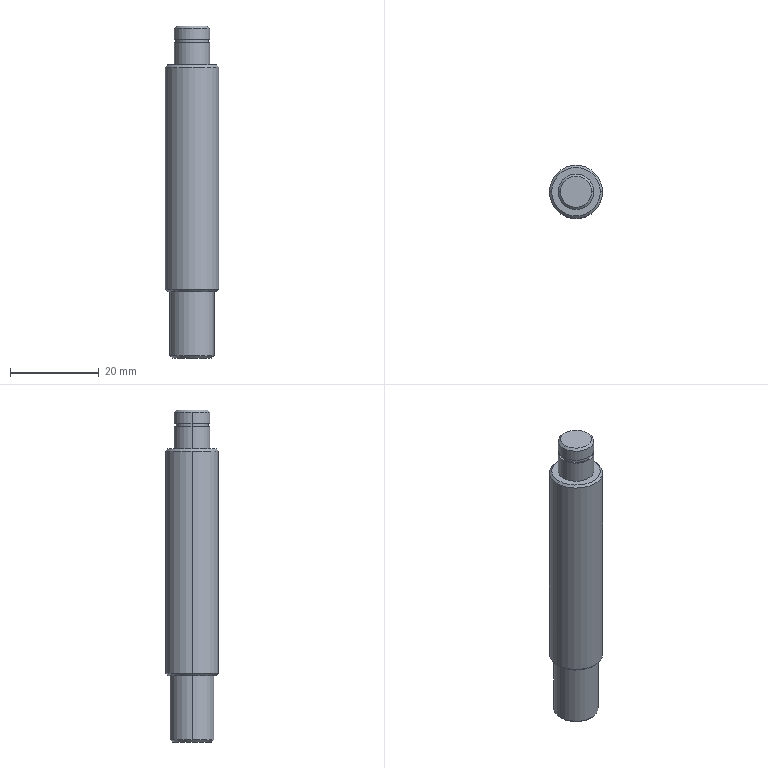Part | STEP file | 06-16 M12 screw rod | 1 solid | 24 faces | box 12 x 12 x 75 mm | volume 7389 mm3 | cylinder 10 | cone 8 | plane 6 | commonest cylinder face diameters 8 x4 7.4 x2 10 x2 12 x2
STEP:
#1=CARTESIAN_POINT('',(0.,0.,0.));
#2=DIRECTION('',(0.,0.,1.));
#3=DIRECTION('',(1.,0.,0.));
#4=AXIS2_PLACEMENT_3D('',#1,#2,#3);
#5=CARTESIAN_POINT('',(-4.5,0.,-75.));
#6=VERTEX_POINT('',#5);
#7=CARTESIAN_POINT('',(4.5,0.,-75.));
#8=VERTEX_POINT('',#7);
#9=CARTESIAN_POINT('',(0.,0.,-75.));
#10=DIRECTION('',(0.,0.,-1.));
#11=DIRECTION('',(1.,0.,0.));
#12=AXIS2_PLACEMENT_3D('',#9,#10,#11);
#13=CIRCLE('',#12,4.5);
#14=CARTESIAN_POINT('',(0.,0.,-75.));
#15=DIRECTION('',(0.,0.,1.));
#16=DIRECTION('',(1.,0.,0.));
#17=AXIS2_PLACEMENT_3D('',#14,#15,#16);
#18=CONICAL_SURFACE('',#17,4.5,0.7854);
#19=CARTESIAN_POINT('',(6.283,0.));
#20=DIRECTION('',(-1.,0.));
#21=VECTOR('',#20,1.);
#22=LINE('',#19,#21);
#23=(GEOMETRIC_REPRESENTATION_CONTEXT(2)PARAMETRIC_REPRESENTATION_CONTEXT()REPRESENTATION_CONTEXT('',''));
#24=DEFINITIONAL_REPRESENTATION('',(#22),#23);
#25=PCURVE('',#18,#24);
#26=CARTESIAN_POINT('',(-4.554,4.554,-75.));
#27=DIRECTION('',(0.,0.,1.));
#28=DIRECTION('',(0.,-1.,0.));
#29=AXIS2_PLACEMENT_3D('',#26,#27,#28);
#30=PLANE('',#29);
#31=CARTESIAN_POINT('',(4.554,9.054));
#32=CARTESIAN_POINT('',(12.348,9.054));
#33=CARTESIAN_POINT('',(8.451,2.304));
#34=CARTESIAN_POINT('',(4.554,-4.446));
#35=CARTESIAN_POINT('',(0.6569,2.304));
#36=CARTESIAN_POINT('',(-3.24,9.054));
#37=CARTESIAN_POINT('',(4.554,9.054));
#38=(BOUNDED_CURVE()B_SPLINE_CURVE(2,(#31,#32,#33,#34,#35,#36,#37),.UNSPECIFIED.,.T.,.F.)B_SPLINE_CURVE_WITH_KNOTS((1,2,2,2,2,1),(-2.094,0.,2.094,4.189,6.283,8.378),.UNSPECIFIED.)CURVE()GEOMETRIC_REPRESENTATION_ITEM()RATIONAL_B_SPLINE_CURVE((1.,0.5,1.,0.5,1.,0.5,1.))REPRESENTATION_ITEM(''));
#39=(GEOMETRIC_REPRESENTATION_CONTEXT(2)PARAMETRIC_REPRESENTATION_CONTEXT()REPRESENTATION_CONTEXT('',''));
#40=DEFINITIONAL_REPRESENTATION('',(#38),#39);
#41=PCURVE('',#30,#40);
#42=SURFACE_CURVE('',#13,(#25,#41),.PCURVE_S1.);
#43=EDGE_CURVE('',#6,#8,#42,.T.);
#44=ORIENTED_EDGE('',*,*,#43,.F.);
#45=CARTESIAN_POINT('',(-5.,0.,-74.5));
#46=VERTEX_POINT('',#45);
#47=CARTESIAN_POINT('',(-4.5,0.,-75.));
#48=DIRECTION('',(-0.7071,0.,0.7071));
#49=VECTOR('',#48,1.);
#50=LINE('',#47,#49);
#51=CARTESIAN_POINT('',(3.142,0.));
#52=DIRECTION('',(0.,1.));
#53=VECTOR('',#52,1.);
#54=LINE('',#51,#53);
#55=(GEOMETRIC_REPRESENTATION_CONTEXT(2)PARAMETRIC_REPRESENTATION_CONTEXT()REPRESENTATION_CONTEXT('',''));
#56=DEFINITIONAL_REPRESENTATION('',(#54),#55);
#57=PCURVE('',#18,#56);
#58=CARTESIAN_POINT('',(0.,0.,-75.));
#59=DIRECTION('',(0.,0.,1.));
#60=DIRECTION('',(1.,0.,0.));
#61=AXIS2_PLACEMENT_3D('',#58,#59,#60);
#62=CONICAL_SURFACE('',#61,4.5,0.7854);
#63=CARTESIAN_POINT('',(3.142,0.));
#64=DIRECTION('',(0.,1.));
#65=VECTOR('',#64,1.);
#66=LINE('',#63,#65);
#67=(GEOMETRIC_REPRESENTATION_CONTEXT(2)PARAMETRIC_REPRESENTATION_CONTEXT()REPRESENTATION_CONTEXT('',''));
#68=DEFINITIONAL_REPRESENTATION('',(#66),#67);
#69=PCURVE('',#62,#68);
#70=SURFACE_CURVE('',#50,(#57,#69),.PCURVE_S1.);
#71=EDGE_CURVE('',#6,#46,#70,.T.);
#72=ORIENTED_EDGE('',*,*,#71,.T.);
#73=CARTESIAN_POINT('',(5.,0.,-74.5));
#74=VERTEX_POINT('',#73);
#75=CARTESIAN_POINT('',(0.,0.,-74.5));
#76=DIRECTION('',(0.,0.,1.));
#77=DIRECTION('',(0.,-1.,0.));
#78=AXIS2_PLACEMENT_3D('',#75,#76,#77);
#79=CIRCLE('',#78,5.);
#80=CARTESIAN_POINT('',(-1.571,0.5));
#81=DIRECTION('',(1.,0.));
#82=VECTOR('',#81,1.);
#83=LINE('',#80,#82);
#84=(GEOMETRIC_REPRESENTATION_CONTEXT(2)PARAMETRIC_REPRESENTATION_CONTEXT()REPRESENTATION_CONTEXT('',''));
#85=DEFINITIONAL_REPRESENTATION('',(#83),#84);
#86=PCURVE('',#18,#85);
#87=CARTESIAN_POINT('',(0.,0.,-74.5));
#88=DIRECTION('',(0.,0.,1.));
#89=DIRECTION('',(1.,0.,0.));
#90=AXIS2_PLACEMENT_3D('',#87,#88,#89);
#91=CYLINDRICAL_SURFACE('',#90,5.);
#92=CARTESIAN_POINT('',(-1.571,0.));
#93=DIRECTION('',(1.,0.));
#94=VECTOR('',#93,1.);
#95=LINE('',#92,#94);
#96=(GEOMETRIC_REPRESENTATION_CONTEXT(2)PARAMETRIC_REPRESENTATION_CONTEXT()REPRESENTATION_CONTEXT('',''));
#97=DEFINITIONAL_REPRESENTATION('',(#95),#96);
#98=PCURVE('',#91,#97);
#99=SURFACE_CURVE('',#79,(#86,#98),.PCURVE_S1.);
#100=EDGE_CURVE('',#74,#46,#99,.T.);
#101=ORIENTED_EDGE('',*,*,#100,.F.);
#102=CARTESIAN_POINT('',(4.5,0.,-75.));
#103=DIRECTION('',(0.7071,0.,0.7071));
#104=VECTOR('',#103,1.);
#105=LINE('',#102,#104);
#106=CARTESIAN_POINT('',(0.,0.));
#107=DIRECTION('',(0.,1.));
#108=VECTOR('',#107,1.);
#109=LINE('',#106,#108);
#110=(GEOMETRIC_REPRESENTATION_CONTEXT(2)PARAMETRIC_REPRESENTATION_CONTEXT()REPRESENTATION_CONTEXT('',''));
#111=DEFINITIONAL_REPRESENTATION('',(#109),#110);
#112=PCURVE('',#18,#111);
#113=CARTESIAN_POINT('',(6.283,0.));
#114=DIRECTION('',(0.,1.));
#115=VECTOR('',#114,1.);
#116=LINE('',#113,#115);
#117=(GEOMETRIC_REPRESENTATION_CONTEXT(2)PARAMETRIC_REPRESENTATION_CONTEXT()REPRESENTATION_CONTEXT('',''));
#118=DEFINITIONAL_REPRESENTATION('',(#116),#117);
#119=PCURVE('',#62,#118);
#120=SURFACE_CURVE('',#105,(#112,#119),.PCURVE_S1.);
#121=EDGE_CURVE('',#8,#74,#120,.T.);
#122=ORIENTED_EDGE('',*,*,#121,.F.);
#123=EDGE_LOOP('',(#44,#72,#101,#122));
#124=FACE_BOUND('',#123,.T.);
#125=ADVANCED_FACE('',(#124),#18,.T.);
#126=ORIENTED_EDGE('',*,*,#100,.T.);
#127=CARTESIAN_POINT('',(-5.,0.,-60.));
#128=VERTEX_POINT('',#127);
#129=CARTESIAN_POINT('',(-5.,0.,-74.5));
#130=DIRECTION('',(0.,0.,1.));
#131=VECTOR('',#130,1.);
#132=LINE('',#129,#131);
#133=CARTESIAN_POINT('',(3.142,0.));
#134=DIRECTION('',(0.,1.));
#135=VECTOR('',#134,1.);
#136=LINE('',#133,#135);
#137=(GEOMETRIC_REPRESENTATION_CONTEXT(2)PARAMETRIC_REPRESENTATION_CONTEXT()REPRESENTATION_CONTEXT('',''));
#138=DEFINITIONAL_REPRESENTATION('',(#136),#137);
#139=PCURVE('',#91,#138);
#140=CARTESIAN_POINT('',(0.,0.,-74.5));
#141=DIRECTION('',(0.,0.,1.));
#142=DIRECTION('',(1.,0.,0.));
#143=AXIS2_PLACEMENT_3D('',#140,#141,#142);
#144=CYLINDRICAL_SURFACE('',#143,5.);
#145=CARTESIAN_POINT('',(3.142,0.));
#146=DIRECTION('',(0.,1.));
#147=VECTOR('',#146,1.);
#148=LINE('',#145,#147);
#149=(GEOMETRIC_REPRESENTATION_CONTEXT(2)PARAMETRIC_REPRESENTATION_CONTEXT()REPRESENTATION_CONTEXT('',''));
#150=DEFINITIONAL_REPRESENTATION('',(#148),#149);
#151=PCURVE('',#144,#150);
#152=SURFACE_CURVE('',#132,(#139,#151),.PCURVE_S1.);
#153=EDGE_CURVE('',#46,#128,#152,.T.);
#154=ORIENTED_EDGE('',*,*,#153,.T.);
#155=CARTESIAN_POINT('',(5.,0.,-60.));
#156=VERTEX_POINT('',#155);
#157=CARTESIAN_POINT('',(0.,0.,-60.));
#158=DIRECTION('',(0.,0.,1.));
#159=DIRECTION('',(1.,0.,0.));
#160=AXIS2_PLACEMENT_3D('',#157,#158,#159);
#161=CIRCLE('',#160,5.);
#162=CARTESIAN_POINT('',(0.,14.5));
#163=DIRECTION('',(1.,0.));
#164=VECTOR('',#163,1.);
#165=LINE('',#162,#164);
#166=(GEOMETRIC_REPRESENTATION_CONTEXT(2)PARAMETRIC_REPRESENTATION_CONTEXT()REPRESENTATION_CONTEXT('',''));
#167=DEFINITIONAL_REPRESENTATION('',(#165),#166);
#168=PCURVE('',#91,#167);
#169=CARTESIAN_POINT('',(-5.566,5.566,-60.));
#170=DIRECTION('',(0.,0.,1.));
#171=DIRECTION('',(0.,-1.,0.));
#172=AXIS2_PLACEMENT_3D('',#169,#170,#171);
#173=PLANE('',#172);
#174=CARTESIAN_POINT('',(5.566,5.566));
#175=DIRECTION('',(0.,1.));
#176=AXIS2_PLACEMENT_2D('',#174,#175);
#177=CIRCLE('',#176,5.);
#178=(GEOMETRIC_REPRESENTATION_CONTEXT(2)PARAMETRIC_REPRESENTATION_CONTEXT()REPRESENTATION_CONTEXT('',''));
#179=DEFINITIONAL_REPRESENTATION('',(#177),#178);
#180=PCURVE('',#173,#179);
#181=SURFACE_CURVE('',#161,(#168,#180),.PCURVE_S1.);
#182=EDGE_CURVE('',#156,#128,#181,.T.);
#183=ORIENTED_EDGE('',*,*,#182,.F.);
#184=CARTESIAN_POINT('',(5.,0.,-74.5));
#185=DIRECTION('',(0.,0.,1.));
#186=VECTOR('',#185,1.);
#187=LINE('',#184,#186);
#188=CARTESIAN_POINT('',(0.,0.));
#189=DIRECTION('',(0.,1.));
#190=VECTOR('',#189,1.);
#191=LINE('',#188,#190);
#192=(GEOMETRIC_REPRESENTATION_CONTEXT(2)PARAMETRIC_REPRESENTATION_CONTEXT()REPRESENTATION_CONTEXT('',''));
#193=DEFINITIONAL_REPRESENTATION('',(#191),#192);
#194=PCURVE('',#91,#193);
#195=CARTESIAN_POINT('',(6.283,0.));
#196=DIRECTION('',(0.,1.));
#197=VECTOR('',#196,1.);
#198=LINE('',#195,#197);
#199=(GEOMETRIC_REPRESENTATION_CONTEXT(2)PARAMETRIC_REPRESENTATION_CONTEXT()REPRESENTATION_CONTEXT('',''));
#200=DEFINITIONAL_REPRESENTATION('',(#198),#199);
#201=PCURVE('',#144,#200);
#202=SURFACE_CURVE('',#187,(#194,#201),.PCURVE_S1.);
#203=EDGE_CURVE('',#74,#156,#202,.T.);
#204=ORIENTED_EDGE('',*,*,#203,.F.);
#205=EDGE_LOOP('',(#126,#154,#183,#204));
#206=FACE_BOUND('',#205,.T.);
#207=ADVANCED_FACE('',(#206),#91,.T.);
#208=CARTESIAN_POINT('',(5.5,0.,-60.));
#209=VERTEX_POINT('',#208);
#210=CARTESIAN_POINT('',(-5.5,0.,-60.));
#211=VERTEX_POINT('',#210);
#212=CARTESIAN_POINT('',(0.,0.,-60.));
#213=DIRECTION('',(0.,0.,1.));
#214=DIRECTION('',(1.,0.,0.));
#215=AXIS2_PLACEMENT_3D('',#212,#213,#214);
#216=CIRCLE('',#215,5.5);
#217=CARTESIAN_POINT('',(0.,0.,-60.));
#218=DIRECTION('',(0.,0.,1.));
#219=DIRECTION('',(1.,0.,0.));
#220=AXIS2_PLACEMENT_3D('',#217,#218,#219);
#221=CONICAL_SURFACE('',#220,5.5,0.7854);
#222=CARTESIAN_POINT('',(0.,0.));
#223=DIRECTION('',(1.,0.));
#224=VECTOR('',#223,1.);
#225=LINE('',#222,#224);
#226=(GEOMETRIC_REPRESENTATION_CONTEXT(2)PARAMETRIC_REPRESENTATION_CONTEXT()REPRESENTATION_CONTEXT('',''));
#227=DEFINITIONAL_REPRESENTATION('',(#225),#226);
#228=PCURVE('',#221,#227);
#229=CARTESIAN_POINT('',(5.566,5.566));
#230=DIRECTION('',(0.,1.));
#231=AXIS2_PLACEMENT_2D('',#229,#230);
#232=CIRCLE('',#231,5.5);
#233=(GEOMETRIC_REPRESENTATION_CONTEXT(2)PARAMETRIC_REPRESENTATION_CONTEXT()REPRESENTATION_CONTEXT('',''));
#234=DEFINITIONAL_REPRESENTATION('',(#232),#233);
#235=PCURVE('',#173,#234);
#236=SURFACE_CURVE('',#216,(#228,#235),.PCURVE_S1.);
#237=EDGE_CURVE('',#209,#211,#236,.T.);
#238=ORIENTED_EDGE('',*,*,#237,.T.);
#239=CARTESIAN_POINT('',(-6.,0.,-59.5));
#240=VERTEX_POINT('',#239);
#241=CARTESIAN_POINT('',(-5.5,0.,-60.));
#242=DIRECTION('',(-0.7071,0.,0.7071));
#243=VECTOR('',#242,1.);
#244=LINE('',#241,#243);
#245=CARTESIAN_POINT('',(3.142,0.));
#246=DIRECTION('',(0.,1.));
#247=VECTOR('',#246,1.);
#248=LINE('',#245,#247);
#249=(GEOMETRIC_REPRESENTATION_CONTEXT(2)PARAMETRIC_REPRESENTATION_CONTEXT()REPRESENTATION_CONTEXT('',''));
#250=DEFINITIONAL_REPRESENTATION('',(#248),#249);
#251=PCURVE('',#221,#250);
#252=CARTESIAN_POINT('',(0.,0.,-60.));
#253=DIRECTION('',(0.,0.,1.));
#254=DIRECTION('',(1.,0.,0.));
#255=AXIS2_PLACEMENT_3D('',#252,#253,#254);
#256=CONICAL_SURFACE('',#255,5.5,0.7854);
#257=CARTESIAN_POINT('',(3.142,0.));
#258=DIRECTION('',(0.,1.));
#259=VECTOR('',#258,1.);
#260=LINE('',#257,#259);
#261=(GEOMETRIC_REPRESENTATION_CONTEXT(2)PARAMETRIC_REPRESENTATION_CONTEXT()REPRESENTATION_CONTEXT('',''));
#262=DEFINITIONAL_REPRESENTATION('',(#260),#261);
#263=PCURVE('',#256,#262);
#264=SURFACE_CURVE('',#244,(#251,#263),.PCURVE_S1.);
#265=EDGE_CURVE('',#211,#240,#264,.T.);
#266=ORIENTED_EDGE('',*,*,#265,.T.);
#267=CARTESIAN_POINT('',(6.,0.,-59.5));
#268=VERTEX_POINT('',#267);
#269=CARTESIAN_POINT('',(0.,0.,-59.5));
#270=DIRECTION('',(0.,0.,1.));
#271=DIRECTION('',(0.,-1.,0.));
#272=AXIS2_PLACEMENT_3D('',#269,#270,#271);
#273=CIRCLE('',#272,6.);
#274=CARTESIAN_POINT('',(-1.571,0.5));
#275=DIRECTION('',(1.,0.));
#276=VECTOR('',#275,1.);
#277=LINE('',#274,#276);
#278=(GEOMETRIC_REPRESENTATION_CONTEXT(2)PARAMETRIC_REPRESENTATION_CONTEXT()REPRESENTATION_CONTEXT('',''));
#279=DEFINITIONAL_REPRESENTATION('',(#277),#278);
#280=PCURVE('',#221,#279);
#281=CARTESIAN_POINT('',(0.,0.,-59.5));
#282=DIRECTION('',(0.,0.,1.));
#283=DIRECTION('',(1.,0.,0.));
#284=AXIS2_PLACEMENT_3D('',#281,#282,#283);
#285=CYLINDRICAL_SURFACE('',#284,6.);
#286=CARTESIAN_POINT('',(-1.571,0.));
#287=DIRECTION('',(1.,0.));
#288=VECTOR('',#287,1.);
#289=LINE('',#286,#288);
#290=(GEOMETRIC_REPRESENTATION_CONTEXT(2)PARAMETRIC_REPRESENTATION_CONTEXT()REPRESENTATION_CONTEXT('',''));
#291=DEFINITIONAL_REPRESENTATION('',(#289),#290);
#292=PCURVE('',#285,#291);
#293=SURFACE_CURVE('',#273,(#280,#292),.PCURVE_S1.);
#294=EDGE_CURVE('',#268,#240,#293,.T.);
#295=ORIENTED_EDGE('',*,*,#294,.F.);
#296=CARTESIAN_POINT('',(5.5,0.,-60.));
#297=DIRECTION('',(0.7071,0.,0.7071));
#298=VECTOR('',#297,1.);
#299=LINE('',#296,#298);
#300=CARTESIAN_POINT('',(0.,0.));
#301=DIRECTION('',(0.,1.));
#302=VECTOR('',#301,1.);
#303=LINE('',#300,#302);
#304=(GEOMETRIC_REPRESENTATION_CONTEXT(2)PARAMETRIC_REPRESENTATION_CONTEXT()REPRESENTATION_CONTEXT('',''));
#305=DEFINITIONAL_REPRESENTATION('',(#303),#304);
#306=PCURVE('',#221,#305);
#307=CARTESIAN_POINT('',(6.283,0.));
#308=DIRECTION('',(0.,1.));
#309=VECTOR('',#308,1.);
#310=LINE('',#307,#309);
#311=(GEOMETRIC_REPRESENTATION_CONTEXT(2)PARAMETRIC_REPRESENTATION_CONTEXT()REPRESENTATION_CONTEXT('',''));
#312=DEFINITIONAL_REPRESENTATION('',(#310),#311);
#313=PCURVE('',#256,#312);
#314=SURFACE_CURVE('',#299,(#306,#313),.PCURVE_S1.);
#315=EDGE_CURVE('',#209,#268,#314,.T.);
#316=ORIENTED_EDGE('',*,*,#315,.F.);
#317=EDGE_LOOP('',(#238,#266,#295,#316));
#318=FACE_BOUND('',#317,.T.);
#319=ADVANCED_FACE('',(#318),#221,.T.);
#320=ORIENTED_EDGE('',*,*,#294,.T.);
#321=CARTESIAN_POINT('',(-6.,0.,-9.3));
#322=VERTEX_POINT('',#321);
#323=CARTESIAN_POINT('',(-6.,0.,-59.5));
#324=DIRECTION('',(0.,0.,1.));
#325=VECTOR('',#324,1.);
#326=LINE('',#323,#325);
#327=CARTESIAN_POINT('',(3.142,0.));
#328=DIRECTION('',(0.,1.));
#329=VECTOR('',#328,1.);
#330=LINE('',#327,#329);
#331=(GEOMETRIC_REPRESENTATION_CONTEXT(2)PARAMETRIC_REPRESENTATION_CONTEXT()REPRESENTATION_CONTEXT('',''));
#332=DEFINITIONAL_REPRESENTATION('',(#330),#331);
#333=PCURVE('',#285,#332);
#334=CARTESIAN_POINT('',(0.,0.,-59.5));
#335=DIRECTION('',(0.,0.,1.));
#336=DIRECTION('',(1.,0.,0.));
#337=AXIS2_PLACEMENT_3D('',#334,#335,#336);
#338=CYLINDRICAL_SURFACE('',#337,6.);
#339=CARTESIAN_POINT('',(3.142,0.));
#340=DIRECTION('',(0.,1.));
#341=VECTOR('',#340,1.);
#342=LINE('',#339,#341);
#343=(GEOMETRIC_REPRESENTATION_CONTEXT(2)PARAMETRIC_REPRESENTATION_CONTEXT()REPRESENTATION_CONTEXT('',''));
#344=DEFINITIONAL_REPRESENTATION('',(#342),#343);
#345=PCURVE('',#338,#344);
#346=SURFACE_CURVE('',#326,(#333,#345),.PCURVE_S1.);
#347=EDGE_CURVE('',#240,#322,#346,.T.);
#348=ORIENTED_EDGE('',*,*,#347,.T.);
#349=CARTESIAN_POINT('',(6.,0.,-9.3));
#350=VERTEX_POINT('',#349);
#351=CARTESIAN_POINT('',(0.,0.,-9.3));
#352=DIRECTION('',(0.,0.,1.));
#353=DIRECTION('',(0.,-1.,0.));
#354=AXIS2_PLACEMENT_3D('',#351,#352,#353);
#355=CIRCLE('',#354,6.);
#356=CARTESIAN_POINT('',(-1.571,50.2));
#357=DIRECTION('',(1.,0.));
#358=VECTOR('',#357,1.);
#359=LINE('',#356,#358);
#360=(GEOMETRIC_REPRESENTATION_CONTEXT(2)PARAMETRIC_REPRESENTATION_CONTEXT()REPRESENTATION_CONTEXT('',''));
#361=DEFINITIONAL_REPRESENTATION('',(#359),#360);
#362=PCURVE('',#285,#361);
#363=CARTESIAN_POINT('',(0.,0.,-8.8));
#364=DIRECTION('',(0.,0.,-1.));
#365=DIRECTION('',(-1.,0.,0.));
#366=AXIS2_PLACEMENT_3D('',#363,#364,#365);
#367=CONICAL_SURFACE('',#366,5.5,0.7854);
#368=CARTESIAN_POINT('',(4.712,0.5));
#369=DIRECTION('',(-1.,0.));
#370=VECTOR('',#369,1.);
#371=LINE('',#368,#370);
#372=(GEOMETRIC_REPRESENTATION_CONTEXT(2)PARAMETRIC_REPRESENTATION_CONTEXT()REPRESENTATION_CONTEXT('',''));
#373=DEFINITIONAL_REPRESENTATION('',(#371),#372);
#374=PCURVE('',#367,#373);
#375=SURFACE_CURVE('',#355,(#362,#374),.PCURVE_S1.);
#376=EDGE_CURVE('',#350,#322,#375,.T.);
#377=ORIENTED_EDGE('',*,*,#376,.F.);
#378=CARTESIAN_POINT('',(6.,0.,-59.5));
#379=DIRECTION('',(0.,0.,1.));
#380=VECTOR('',#379,1.);
#381=LINE('',#378,#380);
#382=CARTESIAN_POINT('',(0.,0.));
#383=DIRECTION('',(0.,1.));
#384=VECTOR('',#383,1.);
#385=LINE('',#382,#384);
#386=(GEOMETRIC_REPRESENTATION_CONTEXT(2)PARAMETRIC_REPRESENTATION_CONTEXT()REPRESENTATION_CONTEXT('',''));
#387=DEFINITIONAL_REPRESENTATION('',(#385),#386);
#388=PCURVE('',#285,#387);
#389=CARTESIAN_POINT('',(6.283,0.));
#390=DIRECTION('',(0.,1.));
#391=VECTOR('',#390,1.);
#392=LINE('',#389,#391);
#393=(GEOMETRIC_REPRESENTATION_CONTEXT(2)PARAMETRIC_REPRESENTATION_CONTEXT()REPRESENTATION_CONTEXT('',''));
#394=DEFINITIONAL_REPRESENTATION('',(#392),#393);
#395=PCURVE('',#338,#394);
#396=SURFACE_CURVE('',#381,(#388,#395),.PCURVE_S1.);
#397=EDGE_CURVE('',#268,#350,#396,.T.);
#398=ORIENTED_EDGE('',*,*,#397,.F.);
#399=EDGE_LOOP('',(#320,#348,#377,#398));
#400=FACE_BOUND('',#399,.T.);
#401=ADVANCED_FACE('',(#400),#285,.T.);
#402=CARTESIAN_POINT('',(5.5,0.,-8.8));
#403=VERTEX_POINT('',#402);
#404=CARTESIAN_POINT('',(-5.5,0.,-8.8));
#405=VERTEX_POINT('',#404);
#406=CARTESIAN_POINT('',(0.,0.,-8.8));
#407=DIRECTION('',(0.,0.,1.));
#408=DIRECTION('',(-1.,0.,0.));
#409=AXIS2_PLACEMENT_3D('',#406,#407,#408);
#410=CIRCLE('',#409,5.5);
#411=CARTESIAN_POINT('',(6.283,0.));
#412=DIRECTION('',(-1.,0.));
#413=VECTOR('',#412,1.);
#414=LINE('',#411,#413);
#415=(GEOMETRIC_REPRESENTATION_CONTEXT(2)PARAMETRIC_REPRESENTATION_CONTEXT()REPRESENTATION_CONTEXT('',''));
#416=DEFINITIONAL_REPRESENTATION('',(#414),#415);
#417=PCURVE('',#367,#416);
#418=CARTESIAN_POINT('',(-5.566,-5.566,-8.8));
#419=DIRECTION('',(0.,0.,-1.));
#420=DIRECTION('',(0.,1.,0.));
#421=AXIS2_PLACEMENT_3D('',#418,#419,#420);
#422=PLANE('',#421);
#423=CARTESIAN_POINT('',(5.566,0.066));
#424=CARTESIAN_POINT('',(-3.96,0.066));
#425=CARTESIAN_POINT('',(0.8029,8.316));
#426=CARTESIAN_POINT('',(5.566,16.566));
#427=CARTESIAN_POINT('',(10.329,8.316));
#428=CARTESIAN_POINT('',(15.092,0.066));
#429=CARTESIAN_POINT('',(5.566,0.066));
#430=(BOUNDED_CURVE()B_SPLINE_CURVE(2,(#423,#424,#425,#426,#427,#428,#429),.UNSPECIFIED.,.T.,.F.)B_SPLINE_CURVE_WITH_KNOTS((1,2,2,2,2,1),(-2.094,0.,2.094,4.189,6.283,8.378),.UNSPECIFIED.)CURVE()GEOMETRIC_REPRESENTATION_ITEM()RATIONAL_B_SPLINE_CURVE((1.,0.5,1.,0.5,1.,0.5,1.))REPRESENTATION_ITEM(''));
#431=(GEOMETRIC_REPRESENTATION_CONTEXT(2)PARAMETRIC_REPRESENTATION_CONTEXT()REPRESENTATION_CONTEXT('',''));
#432=DEFINITIONAL_REPRESENTATION('',(#430),#431);
#433=PCURVE('',#422,#432);
#434=SURFACE_CURVE('',#410,(#417,#433),.PCURVE_S1.);
#435=EDGE_CURVE('',#403,#405,#434,.T.);
#436=ORIENTED_EDGE('',*,*,#435,.F.);
#437=CARTESIAN_POINT('',(5.5,0.,-8.8));
#438=DIRECTION('',(0.7071,0.,-0.7071));
#439=VECTOR('',#438,1.);
#440=LINE('',#437,#439);
#441=CARTESIAN_POINT('',(3.142,0.));
#442=DIRECTION('',(0.,1.));
#443=VECTOR('',#442,1.);
#444=LINE('',#441,#443);
#445=(GEOMETRIC_REPRESENTATION_CONTEXT(2)PARAMETRIC_REPRESENTATION_CONTEXT()REPRESENTATION_CONTEXT('',''));
#446=DEFINITIONAL_REPRESENTATION('',(#444),#445);
#447=PCURVE('',#367,#446);
#448=CARTESIAN_POINT('',(0.,0.,-8.8));
#449=DIRECTION('',(0.,0.,-1.));
#450=DIRECTION('',(-1.,0.,0.));
#451=AXIS2_PLACEMENT_3D('',#448,#449,#450);
#452=CONICAL_SURFACE('',#451,5.5,0.7854);
#453=CARTESIAN_POINT('',(3.142,0.));
#454=DIRECTION('',(0.,1.));
#455=VECTOR('',#454,1.);
#456=LINE('',#453,#455);
#457=(GEOMETRIC_REPRESENTATION_CONTEXT(2)PARAMETRIC_REPRESENTATION_CONTEXT()REPRESENTATION_CONTEXT('',''));
#458=DEFINITIONAL_REPRESENTATION('',(#456),#457);
#459=PCURVE('',#452,#458);
#460=SURFACE_CURVE('',#440,(#447,#459),.PCURVE_S1.);
#461=EDGE_CURVE('',#403,#350,#460,.T.);
#462=ORIENTED_EDGE('',*,*,#461,.T.);
#463=ORIENTED_EDGE('',*,*,#376,.T.);
#464=CARTESIAN_POINT('',(-5.5,0.,-8.8));
#465=DIRECTION('',(-0.7071,0.,-0.7071));
#466=VECTOR('',#465,1.);
#467=LINE('',#464,#466);
#468=CARTESIAN_POINT('',(0.,0.));
#469=DIRECTION('',(0.,1.));
#470=VECTOR('',#469,1.);
#471=LINE('',#468,#470);
#472=(GEOMETRIC_REPRESENTATION_CONTEXT(2)PARAMETRIC_REPRESENTATION_CONTEXT()REPRESENTATION_CONTEXT('',''));
#473=DEFINITIONAL_REPRESENTATION('',(#471),#472);
#474=PCURVE('',#367,#473);
#475=CARTESIAN_POINT('',(6.283,0.));
#476=DIRECTION('',(0.,1.));
#477=VECTOR('',#476,1.);
#478=LINE('',#475,#477);
#479=(GEOMETRIC_REPRESENTATION_CONTEXT(2)PARAMETRIC_REPRESENTATION_CONTEXT()REPRESENTATION_CONTEXT('',''));
#480=DEFINITIONAL_REPRESENTATION('',(#478),#479);
#481=PCURVE('',#452,#480);
#482=SURFACE_CURVE('',#467,(#474,#481),.PCURVE_S1.);
#483=EDGE_CURVE('',#405,#322,#482,.T.);
#484=ORIENTED_EDGE('',*,*,#483,.F.);
#485=EDGE_LOOP('',(#436,#462,#463,#484));
#486=FACE_BOUND('',#485,.T.);
#487=ADVANCED_FACE('',(#486),#367,.T.);
#488=CARTESIAN_POINT('',(4.,0.,-8.8));
#489=VERTEX_POINT('',#488);
#490=CARTESIAN_POINT('',(-4.,0.,-8.8));
#491=VERTEX_POINT('',#490);
#492=CARTESIAN_POINT('',(0.,0.,-8.8));
#493=DIRECTION('',(0.,0.,1.));
#494=DIRECTION('',(1.,0.,0.));
#495=AXIS2_PLACEMENT_3D('',#492,#493,#494);
#496=CIRCLE('',#495,4.);
#497=CARTESIAN_POINT('',(0.,0.,-8.8));
#498=DIRECTION('',(0.,0.,1.));
#499=DIRECTION('',(1.,0.,0.));
#500=AXIS2_PLACEMENT_3D('',#497,#498,#499);
#501=CYLINDRICAL_SURFACE('',#500,4.);
#502=CARTESIAN_POINT('',(0.,0.));
#503=DIRECTION('',(1.,0.));
#504=VECTOR('',#503,1.);
#505=LINE('',#502,#504);
#506=(GEOMETRIC_REPRESENTATION_CONTEXT(2)PARAMETRIC_REPRESENTATION_CONTEXT()REPRESENTATION_CONTEXT('',''));
#507=DEFINITIONAL_REPRESENTATION('',(#505),#506);
#508=PCURVE('',#501,#507);
#509=CARTESIAN_POINT('',(5.566,9.566));
#510=CARTESIAN_POINT('',(12.494,9.566));
#511=CARTESIAN_POINT('',(9.03,3.566));
#512=CARTESIAN_POINT('',(5.566,-2.434));
#513=CARTESIAN_POINT('',(2.102,3.566));
#514=CARTESIAN_POINT('',(-1.362,9.566));
#515=CARTESIAN_POINT('',(5.566,9.566));
#516=(BOUNDED_CURVE()B_SPLINE_CURVE(2,(#509,#510,#511,#512,#513,#514,#515),.UNSPECIFIED.,.T.,.F.)B_SPLINE_CURVE_WITH_KNOTS((1,2,2,2,2,1),(-2.094,0.,2.094,4.189,6.283,8.378),.UNSPECIFIED.)CURVE()GEOMETRIC_REPRESENTATION_ITEM()RATIONAL_B_SPLINE_CURVE((1.,0.5,1.,0.5,1.,0.5,1.))REPRESENTATION_ITEM(''));
#517=(GEOMETRIC_REPRESENTATION_CONTEXT(2)PARAMETRIC_REPRESENTATION_CONTEXT()REPRESENTATION_CONTEXT('',''));
#518=DEFINITIONAL_REPRESENTATION('',(#516),#517);
#519=PCURVE('',#422,#518);
#520=SURFACE_CURVE('',#496,(#508,#519),.PCURVE_S1.);
#521=EDGE_CURVE('',#489,#491,#520,.T.);
#522=ORIENTED_EDGE('',*,*,#521,.T.);
#523=CARTESIAN_POINT('',(-4.,0.,-3.8));
#524=VERTEX_POINT('',#523);
#525=CARTESIAN_POINT('',(-4.,0.,-8.8));
#526=DIRECTION('',(0.,0.,1.));
#527=VECTOR('',#526,1.);
#528=LINE('',#525,#527);
#529=CARTESIAN_POINT('',(3.142,0.));
#530=DIRECTION('',(0.,1.));
#531=VECTOR('',#530,1.);
#532=LINE('',#529,#531);
#533=(GEOMETRIC_REPRESENTATION_CONTEXT(2)PARAMETRIC_REPRESENTATION_CONTEXT()REPRESENTATION_CONTEXT('',''));
#534=DEFINITIONAL_REPRESENTATION('',(#532),#533);
#535=PCURVE('',#501,#534);
#536=CARTESIAN_POINT('',(0.,0.,-8.8));
#537=DIRECTION('',(0.,0.,1.));
#538=DIRECTION('',(1.,0.,0.));
#539=AXIS2_PLACEMENT_3D('',#536,#537,#538);
#540=CYLINDRICAL_SURFACE('',#539,4.);
#541=CARTESIAN_POINT('',(3.142,0.));
#542=DIRECTION('',(0.,1.));
#543=VECTOR('',#542,1.);
#544=LINE('',#541,#543);
#545=(GEOMETRIC_REPRESENTATION_CONTEXT(2)PARAMETRIC_REPRESENTATION_CONTEXT()REPRESENTATION_CONTEXT('',''));
#546=DEFINITIONAL_REPRESENTATION('',(#544),#545);
#547=PCURVE('',#540,#546);
#548=SURFACE_CURVE('',#528,(#535,#547),.PCURVE_S1.);
#549=EDGE_CURVE('',#491,#524,#548,.T.);
#550=ORIENTED_EDGE('',*,*,#549,.T.);
#551=CARTESIAN_POINT('',(4.,0.,-3.8));
#552=VERTEX_POINT('',#551);
#553=CARTESIAN_POINT('',(0.,0.,-3.8));
#554=DIRECTION('',(0.,0.,1.));
#555=DIRECTION('',(1.,0.,0.));
#556=AXIS2_PLACEMENT_3D('',#553,#554,#555);
#557=CIRCLE('',#556,4.);
#558=CARTESIAN_POINT('',(0.,5.));
#559=DIRECTION('',(1.,0.));
#560=VECTOR('',#559,1.);
#561=LINE('',#558,#560);
#562=(GEOMETRIC_REPRESENTATION_CONTEXT(2)PARAMETRIC_REPRESENTATION_CONTEXT()REPRESENTATION_CONTEXT('',''));
#563=DEFINITIONAL_REPRESENTATION('',(#561),#562);
#564=PCURVE('',#501,#563);
#565=CARTESIAN_POINT('',(-4.048,-4.048,-3.8));
#566=DIRECTION('',(0.,0.,-1.));
#567=DIRECTION('',(0.,1.,0.));
#568=AXIS2_PLACEMENT_3D('',#565,#566,#567);
#569=PLANE('',#568);
#570=CARTESIAN_POINT('',(4.048,8.048));
#571=CARTESIAN_POINT('',(10.976,8.048));
#572=CARTESIAN_POINT('',(7.512,2.048));
#573=CARTESIAN_POINT('',(4.048,-3.952));
#574=CARTESIAN_POINT('',(0.5839,2.048));
#575=CARTESIAN_POINT('',(-2.88,8.048));
#576=CARTESIAN_POINT('',(4.048,8.048));
#577=(BOUNDED_CURVE()B_SPLINE_CURVE(2,(#570,#571,#572,#573,#574,#575,#576),.UNSPECIFIED.,.T.,.F.)B_SPLINE_CURVE_WITH_KNOTS((1,2,2,2,2,1),(-2.094,0.,2.094,4.189,6.283,8.378),.UNSPECIFIED.)CURVE()GEOMETRIC_REPRESENTATION_ITEM()RATIONAL_B_SPLINE_CURVE((1.,0.5,1.,0.5,1.,0.5,1.))REPRESENTATION_ITEM(''));
#578=(GEOMETRIC_REPRESENTATION_CONTEXT(2)PARAMETRIC_REPRESENTATION_CONTEXT()REPRESENTATION_CONTEXT('',''));
#579=DEFINITIONAL_REPRESENTATION('',(#577),#578);
#580=PCURVE('',#569,#579);
#581=SURFACE_CURVE('',#557,(#564,#580),.PCURVE_S1.);
#582=EDGE_CURVE('',#552,#524,#581,.T.);
#583=ORIENTED_EDGE('',*,*,#582,.F.);
#584=CARTESIAN_POINT('',(4.,0.,-8.8));
#585=DIRECTION('',(0.,0.,1.));
#586=VECTOR('',#585,1.);
#587=LINE('',#584,#586);
#588=CARTESIAN_POINT('',(0.,0.));
#589=DIRECTION('',(0.,1.));
#590=VECTOR('',#589,1.);
#591=LINE('',#588,#590);
#592=(GEOMETRIC_REPRESENTATION_CONTEXT(2)PARAMETRIC_REPRESENTATION_CONTEXT()REPRESENTATION_CONTEXT('',''));
#593=DEFINITIONAL_REPRESENTATION('',(#591),#592);
#594=PCURVE('',#501,#593);
#595=CARTESIAN_POINT('',(6.283,0.));
#596=DIRECTION('',(0.,1.));
#597=VECTOR('',#596,1.);
#598=LINE('',#595,#597);
#599=(GEOMETRIC_REPRESENTATION_CONTEXT(2)PARAMETRIC_REPRESENTATION_CONTEXT()REPRESENTATION_CONTEXT('',''));
#600=DEFINITIONAL_REPRESENTATION('',(#598),#599);
#601=PCURVE('',#540,#600);
#602=SURFACE_CURVE('',#587,(#594,#601),.PCURVE_S1.);
#603=EDGE_CURVE('',#489,#552,#602,.T.);
#604=ORIENTED_EDGE('',*,*,#603,.F.);
#605=EDGE_LOOP('',(#522,#550,#583,#604));
#606=FACE_BOUND('',#605,.T.);
#607=ADVANCED_FACE('',(#606),#501,.T.);
#608=CARTESIAN_POINT('',(3.7,0.,-3.8));
#609=VERTEX_POINT('',#608);
#610=CARTESIAN_POINT('',(-3.7,0.,-3.8));
#611=VERTEX_POINT('',#610);
#612=CARTESIAN_POINT('',(0.,0.,-3.8));
#613=DIRECTION('',(0.,0.,1.));
#614=DIRECTION('',(1.,0.,0.));
#615=AXIS2_PLACEMENT_3D('',#612,#613,#614);
#616=CIRCLE('',#615,3.7);
#617=CARTESIAN_POINT('',(0.,0.,-3.8));
#618=DIRECTION('',(0.,0.,1.));
#619=DIRECTION('',(1.,0.,0.));
#620=AXIS2_PLACEMENT_3D('',#617,#618,#619);
#621=CYLINDRICAL_SURFACE('',#620,3.7);
#622=CARTESIAN_POINT('',(0.,0.));
#623=DIRECTION('',(1.,0.));
#624=VECTOR('',#623,1.);
#625=LINE('',#622,#624);
#626=(GEOMETRIC_REPRESENTATION_CONTEXT(2)PARAMETRIC_REPRESENTATION_CONTEXT()REPRESENTATION_CONTEXT('',''));
#627=DEFINITIONAL_REPRESENTATION('',(#625),#626);
#628=PCURVE('',#621,#627);
#629=CARTESIAN_POINT('',(4.048,7.748));
#630=CARTESIAN_POINT('',(10.457,7.748));
#631=CARTESIAN_POINT('',(7.252,2.198));
#632=CARTESIAN_POINT('',(4.048,-3.352));
#633=CARTESIAN_POINT('',(0.8437,2.198));
#634=CARTESIAN_POINT('',(-2.361,7.748));
#635=CARTESIAN_POINT('',(4.048,7.748));
#636=(BOUNDED_CURVE()B_SPLINE_CURVE(2,(#629,#630,#631,#632,#633,#634,#635),.UNSPECIFIED.,.T.,.F.)B_SPLINE_CURVE_WITH_KNOTS((1,2,2,2,2,1),(-2.094,0.,2.094,4.189,6.283,8.378),.UNSPECIFIED.)CURVE()GEOMETRIC_REPRESENTATION_ITEM()RATIONAL_B_SPLINE_CURVE((1.,0.5,1.,0.5,1.,0.5,1.))REPRESENTATION_ITEM(''));
#637=(GEOMETRIC_REPRESENTATION_CONTEXT(2)PARAMETRIC_REPRESENTATION_CONTEXT()REPRESENTATION_CONTEXT('',''));
#638=DEFINITIONAL_REPRESENTATION('',(#636),#637);
#639=PCURVE('',#569,#638);
#640=SURFACE_CURVE('',#616,(#628,#639),.PCURVE_S1.);
#641=EDGE_CURVE('',#609,#611,#640,.T.);
#642=ORIENTED_EDGE('',*,*,#641,.T.);
#643=CARTESIAN_POINT('',(-3.7,0.,-3.));
#644=VERTEX_POINT('',#643);
#645=CARTESIAN_POINT('',(-3.7,0.,-3.8));
#646=DIRECTION('',(0.,0.,1.));
#647=VECTOR('',#646,1.);
#648=LINE('',#645,#647);
#649=CARTESIAN_POINT('',(3.142,0.));
#650=DIRECTION('',(0.,1.));
#651=VECTOR('',#650,1.);
#652=LINE('',#649,#651);
#653=(GEOMETRIC_REPRESENTATION_CONTEXT(2)PARAMETRIC_REPRESENTATION_CONTEXT()REPRESENTATION_CONTEXT('',''));
#654=DEFINITIONAL_REPRESENTATION('',(#652),#653);
#655=PCURVE('',#621,#654);
#656=CARTESIAN_POINT('',(0.,0.,-3.8));
#657=DIRECTION('',(0.,0.,1.));
#658=DIRECTION('',(1.,0.,0.));
#659=AXIS2_PLACEMENT_3D('',#656,#657,#658);
#660=CYLINDRICAL_SURFACE('',#659,3.7);
#661=CARTESIAN_POINT('',(3.142,0.));
#662=DIRECTION('',(0.,1.));
#663=VECTOR('',#662,1.);
#664=LINE('',#661,#663);
#665=(GEOMETRIC_REPRESENTATION_CONTEXT(2)PARAMETRIC_REPRESENTATION_CONTEXT()REPRESENTATION_CONTEXT('',''));
#666=DEFINITIONAL_REPRESENTATION('',(#664),#665);
#667=PCURVE('',#660,#666);
#668=SURFACE_CURVE('',#648,(#655,#667),.PCURVE_S1.);
#669=EDGE_CURVE('',#611,#644,#668,.T.);
#670=ORIENTED_EDGE('',*,*,#669,.T.);
#671=CARTESIAN_POINT('',(3.7,0.,-3.));
#672=VERTEX_POINT('',#671);
#673=CARTESIAN_POINT('',(0.,0.,-3.));
#674=DIRECTION('',(0.,0.,1.));
#675=DIRECTION('',(1.,0.,0.));
#676=AXIS2_PLACEMENT_3D('',#673,#674,#675);
#677=CIRCLE('',#676,3.7);
#678=CARTESIAN_POINT('',(0.,0.8));
#679=DIRECTION('',(1.,0.));
#680=VECTOR('',#679,1.);
#681=LINE('',#678,#680);
#682=(GEOMETRIC_REPRESENTATION_CONTEXT(2)PARAMETRIC_REPRESENTATION_CONTEXT()REPRESENTATION_CONTEXT('',''));
#683=DEFINITIONAL_REPRESENTATION('',(#681),#682);
#684=PCURVE('',#621,#683);
#685=CARTESIAN_POINT('',(-4.048,4.048,-3.));
#686=DIRECTION('',(0.,0.,1.));
#687=DIRECTION('',(0.,-1.,0.));
#688=AXIS2_PLACEMENT_3D('',#685,#686,#687);
#689=PLANE('',#688);
#690=CARTESIAN_POINT('',(4.048,4.048));
#691=DIRECTION('',(0.,1.));
#692=AXIS2_PLACEMENT_2D('',#690,#691);
#693=CIRCLE('',#692,3.7);
#694=(GEOMETRIC_REPRESENTATION_CONTEXT(2)PARAMETRIC_REPRESENTATION_CONTEXT()REPRESENTATION_CONTEXT('',''));
#695=DEFINITIONAL_REPRESENTATION('',(#693),#694);
#696=PCURVE('',#689,#695);
#697=SURFACE_CURVE('',#677,(#684,#696),.PCURVE_S1.);
#698=EDGE_CURVE('',#672,#644,#697,.T.);
#699=ORIENTED_EDGE('',*,*,#698,.F.);
#700=CARTESIAN_POINT('',(3.7,0.,-3.8));
#701=DIRECTION('',(0.,0.,1.));
#702=VECTOR('',#701,1.);
#703=LINE('',#700,#702);
#704=CARTESIAN_POINT('',(0.,0.));
#705=DIRECTION('',(0.,1.));
#706=VECTOR('',#705,1.);
#707=LINE('',#704,#706);
#708=(GEOMETRIC_REPRESENTATION_CONTEXT(2)PARAMETRIC_REPRESENTATION_CONTEXT()REPRESENTATION_CONTEXT('',''));
#709=DEFINITIONAL_REPRESENTATION('',(#707),#708);
#710=PCURVE('',#621,#709);
#711=CARTESIAN_POINT('',(6.283,0.));
#712=DIRECTION('',(0.,1.));
#713=VECTOR('',#712,1.);
#714=LINE('',#711,#713);
#715=(GEOMETRIC_REPRESENTATION_CONTEXT(2)PARAMETRIC_REPRESENTATION_CONTEXT()REPRESENTATION_CONTEXT('',''));
#716=DEFINITIONAL_REPRESENTATION('',(#714),#715);
#717=PCURVE('',#660,#716);
#718=SURFACE_CURVE('',#703,(#710,#717),.PCURVE_S1.);
#719=EDGE_CURVE('',#609,#672,#718,.T.);
#720=ORIENTED_EDGE('',*,*,#719,.F.);
#721=EDGE_LOOP('',(#642,#670,#699,#720));
#722=FACE_BOUND('',#721,.T.);
#723=ADVANCED_FACE('',(#722),#621,.T.);
#724=CARTESIAN_POINT('',(4.,0.,-3.));
#725=VERTEX_POINT('',#724);
#726=CARTESIAN_POINT('',(-4.,0.,-3.));
#727=VERTEX_POINT('',#726);
#728=CARTESIAN_POINT('',(0.,0.,-3.));
#729=DIRECTION('',(0.,0.,1.));
#730=DIRECTION('',(1.,0.,0.));
#731=AXIS2_PLACEMENT_3D('',#728,#729,#730);
#732=CIRCLE('',#731,4.);
#733=CARTESIAN_POINT('',(0.,0.,-3.));
#734=DIRECTION('',(0.,0.,1.));
#735=DIRECTION('',(1.,0.,0.));
#736=AXIS2_PLACEMENT_3D('',#733,#734,#735);
#737=CYLINDRICAL_SURFACE('',#736,4.);
#738=CARTESIAN_POINT('',(0.,0.));
#739=DIRECTION('',(1.,0.));
#740=VECTOR('',#739,1.);
#741=LINE('',#738,#740);
#742=(GEOMETRIC_REPRESENTATION_CONTEXT(2)PARAMETRIC_REPRESENTATION_CONTEXT()REPRESENTATION_CONTEXT('',''));
#743=DEFINITIONAL_REPRESENTATION('',(#741),#742);
#744=PCURVE('',#737,#743);
#745=CARTESIAN_POINT('',(4.048,4.048));
#746=DIRECTION('',(0.,1.));
#747=AXIS2_PLACEMENT_2D('',#745,#746);
#748=CIRCLE('',#747,4.);
#749=(GEOMETRIC_REPRESENTATION_CONTEXT(2)PARAMETRIC_REPRESENTATION_CONTEXT()REPRESENTATION_CONTEXT('',''));
#750=DEFINITIONAL_REPRESENTATION('',(#748),#749);
#751=PCURVE('',#689,#750);
#752=SURFACE_CURVE('',#732,(#744,#751),.PCURVE_S1.);
#753=EDGE_CURVE('',#725,#727,#752,.T.);
#754=ORIENTED_EDGE('',*,*,#753,.T.);
#755=CARTESIAN_POINT('',(-4.,0.,-0.5));
#756=VERTEX_POINT('',#755);
#757=CARTESIAN_POINT('',(-4.,0.,-3.));
#758=DIRECTION('',(0.,0.,1.));
#759=VECTOR('',#758,1.);
#760=LINE('',#757,#759);
#761=CARTESIAN_POINT('',(3.142,0.));
#762=DIRECTION('',(0.,1.));
#763=VECTOR('',#762,1.);
#764=LINE('',#761,#763);
#765=(GEOMETRIC_REPRESENTATION_CONTEXT(2)PARAMETRIC_REPRESENTATION_CONTEXT()REPRESENTATION_CONTEXT('',''));
#766=DEFINITIONAL_REPRESENTATION('',(#764),#765);
#767=PCURVE('',#737,#766);
#768=CARTESIAN_POINT('',(0.,0.,-3.));
#769=DIRECTION('',(0.,0.,1.));
#770=DIRECTION('',(1.,0.,0.));
#771=AXIS2_PLACEMENT_3D('',#768,#769,#770);
#772=CYLINDRICAL_SURFACE('',#771,4.);
#773=CARTESIAN_POINT('',(3.142,0.));
#774=DIRECTION('',(0.,1.));
#775=VECTOR('',#774,1.);
#776=LINE('',#773,#775);
#777=(GEOMETRIC_REPRESENTATION_CONTEXT(2)PARAMETRIC_REPRESENTATION_CONTEXT()REPRESENTATION_CONTEXT('',''));
#778=DEFINITIONAL_REPRESENTATION('',(#776),#777);
#779=PCURVE('',#772,#778);
#780=SURFACE_CURVE('',#760,(#767,#779),.PCURVE_S1.);
#781=EDGE_CURVE('',#727,#756,#780,.T.);
#782=ORIENTED_EDGE('',*,*,#781,.T.);
#783=CARTESIAN_POINT('',(4.,0.,-0.5));
#784=VERTEX_POINT('',#783);
#785=CARTESIAN_POINT('',(0.,0.,-0.5));
#786=DIRECTION('',(0.,0.,1.));
#787=DIRECTION('',(0.,-1.,0.));
#788=AXIS2_PLACEMENT_3D('',#785,#786,#787);
#789=CIRCLE('',#788,4.);
#790=CARTESIAN_POINT('',(-1.571,2.5));
#791=DIRECTION('',(1.,0.));
#792=VECTOR('',#791,1.);
#793=LINE('',#790,#792);
#794=(GEOMETRIC_REPRESENTATION_CONTEXT(2)PARAMETRIC_REPRESENTATION_CONTEXT()REPRESENTATION_CONTEXT('',''));
#795=DEFINITIONAL_REPRESENTATION('',(#793),#794);
#796=PCURVE('',#737,#795);
#797=CARTESIAN_POINT('',(0.,0.,0.));
#798=DIRECTION('',(0.,0.,-1.));
#799=DIRECTION('',(-1.,0.,0.));
#800=AXIS2_PLACEMENT_3D('',#797,#798,#799);
#801=CONICAL_SURFACE('',#800,3.5,0.7854);
#802=CARTESIAN_POINT('',(4.712,0.5));
#803=DIRECTION('',(-1.,0.));
#804=VECTOR('',#803,1.);
#805=LINE('',#802,#804);
#806=(GEOMETRIC_REPRESENTATION_CONTEXT(2)PARAMETRIC_REPRESENTATION_CONTEXT()REPRESENTATION_CONTEXT('',''));
#807=DEFINITIONAL_REPRESENTATION('',(#805),#806);
#808=PCURVE('',#801,#807);
#809=SURFACE_CURVE('',#789,(#796,#808),.PCURVE_S1.);
#810=EDGE_CURVE('',#784,#756,#809,.T.);
#811=ORIENTED_EDGE('',*,*,#810,.F.);
#812=CARTESIAN_POINT('',(4.,0.,-3.));
#813=DIRECTION('',(0.,0.,1.));
#814=VECTOR('',#813,1.);
#815=LINE('',#812,#814);
#816=CARTESIAN_POINT('',(0.,0.));
#817=DIRECTION('',(0.,1.));
#818=VECTOR('',#817,1.);
#819=LINE('',#816,#818);
#820=(GEOMETRIC_REPRESENTATION_CONTEXT(2)PARAMETRIC_REPRESENTATION_CONTEXT()REPRESENTATION_CONTEXT('',''));
#821=DEFINITIONAL_REPRESENTATION('',(#819),#820);
#822=PCURVE('',#737,#821);
#823=CARTESIAN_POINT('',(6.283,0.));
#824=DIRECTION('',(0.,1.));
#825=VECTOR('',#824,1.);
#826=LINE('',#823,#825);
#827=(GEOMETRIC_REPRESENTATION_CONTEXT(2)PARAMETRIC_REPRESENTATION_CONTEXT()REPRESENTATION_CONTEXT('',''));
#828=DEFINITIONAL_REPRESENTATION('',(#826),#827);
#829=PCURVE('',#772,#828);
#830=SURFACE_CURVE('',#815,(#822,#829),.PCURVE_S1.);
#831=EDGE_CURVE('',#725,#784,#830,.T.);
#832=ORIENTED_EDGE('',*,*,#831,.F.);
#833=EDGE_LOOP('',(#754,#782,#811,#832));
#834=FACE_BOUND('',#833,.T.);
#835=ADVANCED_FACE('',(#834),#737,.T.);
#836=CARTESIAN_POINT('',(3.5,0.,0.));
#837=VERTEX_POINT('',#836);
#838=CARTESIAN_POINT('',(-3.5,0.,0.));
#839=VERTEX_POINT('',#838);
#840=CARTESIAN_POINT('',(0.,0.,0.));
#841=DIRECTION('',(0.,0.,1.));
#842=DIRECTION('',(-1.,0.,0.));
#843=AXIS2_PLACEMENT_3D('',#840,#841,#842);
#844=CIRCLE('',#843,3.5);
#845=CARTESIAN_POINT('',(6.283,0.));
#846=DIRECTION('',(-1.,0.));
#847=VECTOR('',#846,1.);
#848=LINE('',#845,#847);
#849=(GEOMETRIC_REPRESENTATION_CONTEXT(2)PARAMETRIC_REPRESENTATION_CONTEXT()REPRESENTATION_CONTEXT('',''));
#850=DEFINITIONAL_REPRESENTATION('',(#848),#849);
#851=PCURVE('',#801,#850);
#852=CARTESIAN_POINT('',(-3.542,-3.542,0.));
#853=DIRECTION('',(0.,0.,-1.));
#854=DIRECTION('',(0.,1.,0.));
#855=AXIS2_PLACEMENT_3D('',#852,#853,#854);
#856=PLANE('',#855);
#857=CARTESIAN_POINT('',(3.542,0.042));
#858=CARTESIAN_POINT('',(-2.52,0.042));
#859=CARTESIAN_POINT('',(0.5109,5.292));
#860=CARTESIAN_POINT('',(3.542,10.542));
#861=CARTESIAN_POINT('',(6.573,5.292));
#862=CARTESIAN_POINT('',(9.604,0.042));
#863=CARTESIAN_POINT('',(3.542,0.042));
#864=(BOUNDED_CURVE()B_SPLINE_CURVE(2,(#857,#858,#859,#860,#861,#862,#863),.UNSPECIFIED.,.T.,.F.)B_SPLINE_CURVE_WITH_KNOTS((1,2,2,2,2,1),(-2.094,0.,2.094,4.189,6.283,8.378),.UNSPECIFIED.)CURVE()GEOMETRIC_REPRESENTATION_ITEM()RATIONAL_B_SPLINE_CURVE((1.,0.5,1.,0.5,1.,0.5,1.))REPRESENTATION_ITEM(''));
#865=(GEOMETRIC_REPRESENTATION_CONTEXT(2)PARAMETRIC_REPRESENTATION_CONTEXT()REPRESENTATION_CONTEXT('',''));
#866=DEFINITIONAL_REPRESENTATION('',(#864),#865);
#867=PCURVE('',#856,#866);
#868=SURFACE_CURVE('',#844,(#851,#867),.PCURVE_S1.);
#869=EDGE_CURVE('',#837,#839,#868,.T.);
#870=ORIENTED_EDGE('',*,*,#869,.F.);
#871=CARTESIAN_POINT('',(3.5,0.,0.));
#872=DIRECTION('',(0.7071,0.,-0.7071));
#873=VECTOR('',#872,1.);
#874=LINE('',#871,#873);
#875=CARTESIAN_POINT('',(3.142,0.));
#876=DIRECTION('',(0.,1.));
#877=VECTOR('',#876,1.);
#878=LINE('',#875,#877);
#879=(GEOMETRIC_REPRESENTATION_CONTEXT(2)PARAMETRIC_REPRESENTATION_CONTEXT()REPRESENTATION_CONTEXT('',''));
#880=DEFINITIONAL_REPRESENTATION('',(#878),#879);
#881=PCURVE('',#801,#880);
#882=CARTESIAN_POINT('',(0.,0.,0.));
#883=DIRECTION('',(0.,0.,-1.));
#884=DIRECTION('',(-1.,0.,0.));
#885=AXIS2_PLACEMENT_3D('',#882,#883,#884);
#886=CONICAL_SURFACE('',#885,3.5,0.7854);
#887=CARTESIAN_POINT('',(3.142,0.));
#888=DIRECTION('',(0.,1.));
#889=VECTOR('',#888,1.);
#890=LINE('',#887,#889);
#891=(GEOMETRIC_REPRESENTATION_CONTEXT(2)PARAMETRIC_REPRESENTATION_CONTEXT()REPRESENTATION_CONTEXT('',''));
#892=DEFINITIONAL_REPRESENTATION('',(#890),#891);
#893=PCURVE('',#886,#892);
#894=SURFACE_CURVE('',#874,(#881,#893),.PCURVE_S1.);
#895=EDGE_CURVE('',#837,#784,#894,.T.);
#896=ORIENTED_EDGE('',*,*,#895,.T.);
#897=ORIENTED_EDGE('',*,*,#810,.T.);
#898=CARTESIAN_POINT('',(-3.5,0.,0.));
#899=DIRECTION('',(-0.7071,0.,-0.7071));
#900=VECTOR('',#899,1.);
#901=LINE('',#898,#900);
#902=CARTESIAN_POINT('',(0.,0.));
#903=DIRECTION('',(0.,1.));
#904=VECTOR('',#903,1.);
#905=LINE('',#902,#904);
#906=(GEOMETRIC_REPRESENTATION_CONTEXT(2)PARAMETRIC_REPRESENTATION_CONTEXT()REPRESENTATION_CONTEXT('',''));
#907=DEFINITIONAL_REPRESENTATION('',(#905),#906);
#908=PCURVE('',#801,#907);
#909=CARTESIAN_POINT('',(6.283,0.));
#910=DIRECTION('',(0.,1.));
#911=VECTOR('',#910,1.);
#912=LINE('',#909,#911);
#913=(GEOMETRIC_REPRESENTATION_CONTEXT(2)PARAMETRIC_REPRESENTATION_CONTEXT()REPRESENTATION_CONTEXT('',''));
#914=DEFINITIONAL_REPRESENTATION('',(#912),#913);
#915=PCURVE('',#886,#914);
#916=SURFACE_CURVE('',#901,(#908,#915),.PCURVE_S1.);
#917=EDGE_CURVE('',#839,#756,#916,.T.);
#918=ORIENTED_EDGE('',*,*,#917,.F.);
#919=EDGE_LOOP('',(#870,#896,#897,#918));
#920=FACE_BOUND('',#919,.T.);
#921=ADVANCED_FACE('',(#920),#801,.T.);
#922=ORIENTED_EDGE('',*,*,#71,.F.);
#923=CARTESIAN_POINT('',(0.,0.,-75.));
#924=DIRECTION('',(0.,0.,-1.));
#925=DIRECTION('',(1.,0.,0.));
#926=AXIS2_PLACEMENT_3D('',#923,#924,#925);
#927=CIRCLE('',#926,4.5);
#928=CARTESIAN_POINT('',(6.283,0.));
#929=DIRECTION('',(-1.,0.));
#930=VECTOR('',#929,1.);
#931=LINE('',#928,#930);
#932=(GEOMETRIC_REPRESENTATION_CONTEXT(2)PARAMETRIC_REPRESENTATION_CONTEXT()REPRESENTATION_CONTEXT('',''));
#933=DEFINITIONAL_REPRESENTATION('',(#931),#932);
#934=PCURVE('',#62,#933);
#935=CARTESIAN_POINT('',(4.554,9.054));
#936=CARTESIAN_POINT('',(12.348,9.054));
#937=CARTESIAN_POINT('',(8.451,2.304));
#938=CARTESIAN_POINT('',(4.554,-4.446));
#939=CARTESIAN_POINT('',(0.6569,2.304));
#940=CARTESIAN_POINT('',(-3.24,9.054));
#941=CARTESIAN_POINT('',(4.554,9.054));
#942=(BOUNDED_CURVE()B_SPLINE_CURVE(2,(#935,#936,#937,#938,#939,#940,#941),.UNSPECIFIED.,.T.,.F.)B_SPLINE_CURVE_WITH_KNOTS((1,2,2,2,2,1),(-2.094,0.,2.094,4.189,6.283,8.378),.UNSPECIFIED.)CURVE()GEOMETRIC_REPRESENTATION_ITEM()RATIONAL_B_SPLINE_CURVE((1.,0.5,1.,0.5,1.,0.5,1.))REPRESENTATION_ITEM(''));
#943=(GEOMETRIC_REPRESENTATION_CONTEXT(2)PARAMETRIC_REPRESENTATION_CONTEXT()REPRESENTATION_CONTEXT('',''));
#944=DEFINITIONAL_REPRESENTATION('',(#942),#943);
#945=PCURVE('',#30,#944);
#946=SURFACE_CURVE('',#927,(#934,#945),.PCURVE_S1.);
#947=EDGE_CURVE('',#8,#6,#946,.T.);
#948=ORIENTED_EDGE('',*,*,#947,.F.);
#949=ORIENTED_EDGE('',*,*,#121,.T.);
#950=CARTESIAN_POINT('',(0.,0.,-74.5));
#951=DIRECTION('',(0.,0.,1.));
#952=DIRECTION('',(0.,-1.,0.));
#953=AXIS2_PLACEMENT_3D('',#950,#951,#952);
#954=CIRCLE('',#953,5.);
#955=CARTESIAN_POINT('',(-1.571,0.5));
#956=DIRECTION('',(1.,0.));
#957=VECTOR('',#956,1.);
#958=LINE('',#955,#957);
#959=(GEOMETRIC_REPRESENTATION_CONTEXT(2)PARAMETRIC_REPRESENTATION_CONTEXT()REPRESENTATION_CONTEXT('',''));
#960=DEFINITIONAL_REPRESENTATION('',(#958),#959);
#961=PCURVE('',#62,#960);
#962=CARTESIAN_POINT('',(-1.571,0.));
#963=DIRECTION('',(1.,0.));
#964=VECTOR('',#963,1.);
#965=LINE('',#962,#964);
#966=(GEOMETRIC_REPRESENTATION_CONTEXT(2)PARAMETRIC_REPRESENTATION_CONTEXT()REPRESENTATION_CONTEXT('',''));
#967=DEFINITIONAL_REPRESENTATION('',(#965),#966);
#968=PCURVE('',#144,#967);
#969=SURFACE_CURVE('',#954,(#961,#968),.PCURVE_S1.);
#970=EDGE_CURVE('',#46,#74,#969,.T.);
#971=ORIENTED_EDGE('',*,*,#970,.F.);
#972=EDGE_LOOP('',(#922,#948,#949,#971));
#973=FACE_BOUND('',#972,.T.);
#974=ADVANCED_FACE('',(#973),#62,.T.);
#975=ORIENTED_EDGE('',*,*,#947,.T.);
#976=ORIENTED_EDGE('',*,*,#43,.T.);
#977=EDGE_LOOP('',(#975,#976));
#978=FACE_BOUND('',#977,.T.);
#979=ADVANCED_FACE('',(#978),#30,.F.);
#980=ORIENTED_EDGE('',*,*,#153,.F.);
#981=ORIENTED_EDGE('',*,*,#970,.T.);
#982=ORIENTED_EDGE('',*,*,#203,.T.);
#983=CARTESIAN_POINT('',(0.,0.,-60.));
#984=DIRECTION('',(0.,0.,1.));
#985=DIRECTION('',(1.,0.,0.));
#986=AXIS2_PLACEMENT_3D('',#983,#984,#985);
#987=CIRCLE('',#986,5.);
#988=CARTESIAN_POINT('',(0.,14.5));
#989=DIRECTION('',(1.,0.));
#990=VECTOR('',#989,1.);
#991=LINE('',#988,#990);
#992=(GEOMETRIC_REPRESENTATION_CONTEXT(2)PARAMETRIC_REPRESENTATION_CONTEXT()REPRESENTATION_CONTEXT('',''));
#993=DEFINITIONAL_REPRESENTATION('',(#991),#992);
#994=PCURVE('',#144,#993);
#995=CARTESIAN_POINT('',(5.566,5.566));
#996=DIRECTION('',(0.,1.));
#997=AXIS2_PLACEMENT_2D('',#995,#996);
#998=CIRCLE('',#997,5.);
#999=(GEOMETRIC_REPRESENTATION_CONTEXT(2)PARAMETRIC_REPRESENTATION_CONTEXT()REPRESENTATION_CONTEXT('',''));
#1000=DEFINITIONAL_REPRESENTATION('',(#998),#999);
#1001=PCURVE('',#173,#1000);
#1002=SURFACE_CURVE('',#987,(#994,#1001),.PCURVE_S1.);
#1003=EDGE_CURVE('',#128,#156,#1002,.T.);
#1004=ORIENTED_EDGE('',*,*,#1003,.F.);
#1005=EDGE_LOOP('',(#980,#981,#982,#1004));
#1006=FACE_BOUND('',#1005,.T.);
#1007=ADVANCED_FACE('',(#1006),#144,.T.);
#1008=ORIENTED_EDGE('',*,*,#182,.T.);
#1009=ORIENTED_EDGE('',*,*,#1003,.T.);
#1010=EDGE_LOOP('',(#1008,#1009));
#1011=FACE_BOUND('',#1010,.T.);
#1012=ORIENTED_EDGE('',*,*,#237,.F.);
#1013=CARTESIAN_POINT('',(0.,0.,-60.));
#1014=DIRECTION('',(0.,0.,1.));
#1015=DIRECTION('',(1.,0.,0.));
#1016=AXIS2_PLACEMENT_3D('',#1013,#1014,#1015);
#1017=CIRCLE('',#1016,5.5);
#1018=CARTESIAN_POINT('',(5.566,5.566));
#1019=DIRECTION('',(0.,1.));
#1020=AXIS2_PLACEMENT_2D('',#1018,#1019);
#1021=CIRCLE('',#1020,5.5);
#1022=(GEOMETRIC_REPRESENTATION_CONTEXT(2)PARAMETRIC_REPRESENTATION_CONTEXT()REPRESENTATION_CONTEXT('',''));
#1023=DEFINITIONAL_REPRESENTATION('',(#1021),#1022);
#1024=PCURVE('',#173,#1023);
#1025=CARTESIAN_POINT('',(0.,0.));
#1026=DIRECTION('',(1.,0.));
#1027=VECTOR('',#1026,1.);
#1028=LINE('',#1025,#1027);
#1029=(GEOMETRIC_REPRESENTATION_CONTEXT(2)PARAMETRIC_REPRESENTATION_CONTEXT()REPRESENTATION_CONTEXT('',''));
#1030=DEFINITIONAL_REPRESENTATION('',(#1028),#1029);
#1031=PCURVE('',#256,#1030);
#1032=SURFACE_CURVE('',#1017,(#1024,#1031),.PCURVE_S1.);
#1033=EDGE_CURVE('',#211,#209,#1032,.T.);
#1034=ORIENTED_EDGE('',*,*,#1033,.F.);
#1035=EDGE_LOOP('',(#1012,#1034));
#1036=FACE_BOUND('',#1035,.T.);
#1037=ADVANCED_FACE('',(#1011,#1036),#173,.F.);
#1038=ORIENTED_EDGE('',*,*,#265,.F.);
#1039=ORIENTED_EDGE('',*,*,#1033,.T.);
#1040=ORIENTED_EDGE('',*,*,#315,.T.);
#1041=CARTESIAN_POINT('',(0.,0.,-59.5));
#1042=DIRECTION('',(0.,0.,1.));
#1043=DIRECTION('',(0.,-1.,0.));
#1044=AXIS2_PLACEMENT_3D('',#1041,#1042,#1043);
#1045=CIRCLE('',#1044,6.);
#1046=CARTESIAN_POINT('',(-1.571,0.5));
#1047=DIRECTION('',(1.,0.));
#1048=VECTOR('',#1047,1.);
#1049=LINE('',#1046,#1048);
#1050=(GEOMETRIC_REPRESENTATION_CONTEXT(2)PARAMETRIC_REPRESENTATION_CONTEXT()REPRESENTATION_CONTEXT('',''));
#1051=DEFINITIONAL_REPRESENTATION('',(#1049),#1050);
#1052=PCURVE('',#256,#1051);
#1053=CARTESIAN_POINT('',(-1.571,0.));
#1054=DIRECTION('',(1.,0.));
#1055=VECTOR('',#1054,1.);
#1056=LINE('',#1053,#1055);
#1057=(GEOMETRIC_REPRESENTATION_CONTEXT(2)PARAMETRIC_REPRESENTATION_CONTEXT()REPRESENTATION_CONTEXT('',''));
#1058=DEFINITIONAL_REPRESENTATION('',(#1056),#1057);
#1059=PCURVE('',#338,#1058);
#1060=SURFACE_CURVE('',#1045,(#1052,#1059),.PCURVE_S1.);
#1061=EDGE_CURVE('',#240,#268,#1060,.T.);
#1062=ORIENTED_EDGE('',*,*,#1061,.F.);
#1063=EDGE_LOOP('',(#1038,#1039,#1040,#1062));
#1064=FACE_BOUND('',#1063,.T.);
#1065=ADVANCED_FACE('',(#1064),#256,.T.);
#1066=ORIENTED_EDGE('',*,*,#347,.F.);
#1067=ORIENTED_EDGE('',*,*,#1061,.T.);
#1068=ORIENTED_EDGE('',*,*,#397,.T.);
#1069=CARTESIAN_POINT('',(0.,0.,-9.3));
#1070=DIRECTION('',(0.,0.,1.));
#1071=DIRECTION('',(0.,-1.,0.));
#1072=AXIS2_PLACEMENT_3D('',#1069,#1070,#1071);
#1073=CIRCLE('',#1072,6.);
#1074=CARTESIAN_POINT('',(-1.571,50.2));
#1075=DIRECTION('',(1.,0.));
#1076=VECTOR('',#1075,1.);
#1077=LINE('',#1074,#1076);
#1078=(GEOMETRIC_REPRESENTATION_CONTEXT(2)PARAMETRIC_REPRESENTATION_CONTEXT()REPRESENTATION_CONTEXT('',''));
#1079=DEFINITIONAL_REPRESENTATION('',(#1077),#1078);
#1080=PCURVE('',#338,#1079);
#1081=CARTESIAN_POINT('',(10.996,0.5));
#1082=DIRECTION('',(-1.,0.));
#1083=VECTOR('',#1082,1.);
#1084=LINE('',#1081,#1083);
#1085=(GEOMETRIC_REPRESENTATION_CONTEXT(2)PARAMETRIC_REPRESENTATION_CONTEXT()REPRESENTATION_CONTEXT('',''));
#1086=DEFINITIONAL_REPRESENTATION('',(#1084),#1085);
#1087=PCURVE('',#452,#1086);
#1088=SURFACE_CURVE('',#1073,(#1080,#1087),.PCURVE_S1.);
#1089=EDGE_CURVE('',#322,#350,#1088,.T.);
#1090=ORIENTED_EDGE('',*,*,#1089,.F.);
#1091=EDGE_LOOP('',(#1066,#1067,#1068,#1090));
#1092=FACE_BOUND('',#1091,.T.);
#1093=ADVANCED_FACE('',(#1092),#338,.T.);
#1094=ORIENTED_EDGE('',*,*,#461,.F.);
#1095=CARTESIAN_POINT('',(0.,0.,-8.8));
#1096=DIRECTION('',(0.,0.,1.));
#1097=DIRECTION('',(-1.,0.,0.));
#1098=AXIS2_PLACEMENT_3D('',#1095,#1096,#1097);
#1099=CIRCLE('',#1098,5.5);
#1100=CARTESIAN_POINT('',(6.283,0.));
#1101=DIRECTION('',(-1.,0.));
#1102=VECTOR('',#1101,1.);
#1103=LINE('',#1100,#1102);
#1104=(GEOMETRIC_REPRESENTATION_CONTEXT(2)PARAMETRIC_REPRESENTATION_CONTEXT()REPRESENTATION_CONTEXT('',''));
#1105=DEFINITIONAL_REPRESENTATION('',(#1103),#1104);
#1106=PCURVE('',#452,#1105);
#1107=CARTESIAN_POINT('',(5.566,0.066));
#1108=CARTESIAN_POINT('',(-3.96,0.066));
#1109=CARTESIAN_POINT('',(0.8029,8.316));
#1110=CARTESIAN_POINT('',(5.566,16.566));
#1111=CARTESIAN_POINT('',(10.329,8.316));
#1112=CARTESIAN_POINT('',(15.092,0.066));
#1113=CARTESIAN_POINT('',(5.566,0.066));
#1114=(BOUNDED_CURVE()B_SPLINE_CURVE(2,(#1107,#1108,#1109,#1110,#1111,#1112,#1113),.UNSPECIFIED.,.T.,.F.)B_SPLINE_CURVE_WITH_KNOTS((1,2,2,2,2,1),(-2.094,0.,2.094,4.189,6.283,8.378),.UNSPECIFIED.)CURVE()GEOMETRIC_REPRESENTATION_ITEM()RATIONAL_B_SPLINE_CURVE((1.,0.5,1.,0.5,1.,0.5,1.))REPRESENTATION_ITEM(''));
#1115=(GEOMETRIC_REPRESENTATION_CONTEXT(2)PARAMETRIC_REPRESENTATION_CONTEXT()REPRESENTATION_CONTEXT('',''));
#1116=DEFINITIONAL_REPRESENTATION('',(#1114),#1115);
#1117=PCURVE('',#422,#1116);
#1118=SURFACE_CURVE('',#1099,(#1106,#1117),.PCURVE_S1.);
#1119=EDGE_CURVE('',#405,#403,#1118,.T.);
#1120=ORIENTED_EDGE('',*,*,#1119,.F.);
#1121=ORIENTED_EDGE('',*,*,#483,.T.);
#1122=ORIENTED_EDGE('',*,*,#1089,.T.);
#1123=EDGE_LOOP('',(#1094,#1120,#1121,#1122));
#1124=FACE_BOUND('',#1123,.T.);
#1125=ADVANCED_FACE('',(#1124),#452,.T.);
#1126=ORIENTED_EDGE('',*,*,#521,.F.);
#1127=CARTESIAN_POINT('',(0.,0.,-8.8));
#1128=DIRECTION('',(0.,0.,1.));
#1129=DIRECTION('',(1.,0.,0.));
#1130=AXIS2_PLACEMENT_3D('',#1127,#1128,#1129);
#1131=CIRCLE('',#1130,4.);
#1132=CARTESIAN_POINT('',(5.566,9.566));
#1133=CARTESIAN_POINT('',(12.494,9.566));
#1134=CARTESIAN_POINT('',(9.03,3.566));
#1135=CARTESIAN_POINT('',(5.566,-2.434));
#1136=CARTESIAN_POINT('',(2.102,3.566));
#1137=CARTESIAN_POINT('',(-1.362,9.566));
#1138=CARTESIAN_POINT('',(5.566,9.566));
#1139=(BOUNDED_CURVE()B_SPLINE_CURVE(2,(#1132,#1133,#1134,#1135,#1136,#1137,#1138),.UNSPECIFIED.,.T.,.F.)B_SPLINE_CURVE_WITH_KNOTS((1,2,2,2,2,1),(-2.094,0.,2.094,4.189,6.283,8.378),.UNSPECIFIED.)CURVE()GEOMETRIC_REPRESENTATION_ITEM()RATIONAL_B_SPLINE_CURVE((1.,0.5,1.,0.5,1.,0.5,1.))REPRESENTATION_ITEM(''));
#1140=(GEOMETRIC_REPRESENTATION_CONTEXT(2)PARAMETRIC_REPRESENTATION_CONTEXT()REPRESENTATION_CONTEXT('',''));
#1141=DEFINITIONAL_REPRESENTATION('',(#1139),#1140);
#1142=PCURVE('',#422,#1141);
#1143=CARTESIAN_POINT('',(0.,0.));
#1144=DIRECTION('',(1.,0.));
#1145=VECTOR('',#1144,1.);
#1146=LINE('',#1143,#1145);
#1147=(GEOMETRIC_REPRESENTATION_CONTEXT(2)PARAMETRIC_REPRESENTATION_CONTEXT()REPRESENTATION_CONTEXT('',''));
#1148=DEFINITIONAL_REPRESENTATION('',(#1146),#1147);
#1149=PCURVE('',#540,#1148);
#1150=SURFACE_CURVE('',#1131,(#1142,#1149),.PCURVE_S1.);
#1151=EDGE_CURVE('',#491,#489,#1150,.T.);
#1152=ORIENTED_EDGE('',*,*,#1151,.F.);
#1153=EDGE_LOOP('',(#1126,#1152));
#1154=FACE_BOUND('',#1153,.T.);
#1155=ORIENTED_EDGE('',*,*,#1119,.T.);
#1156=ORIENTED_EDGE('',*,*,#435,.T.);
#1157=EDGE_LOOP('',(#1155,#1156));
#1158=FACE_BOUND('',#1157,.T.);
#1159=ADVANCED_FACE('',(#1154,#1158),#422,.F.);
#1160=ORIENTED_EDGE('',*,*,#549,.F.);
#1161=ORIENTED_EDGE('',*,*,#1151,.T.);
#1162=ORIENTED_EDGE('',*,*,#603,.T.);
#1163=CARTESIAN_POINT('',(0.,0.,-3.8));
#1164=DIRECTION('',(0.,0.,1.));
#1165=DIRECTION('',(1.,0.,0.));
#1166=AXIS2_PLACEMENT_3D('',#1163,#1164,#1165);
#1167=CIRCLE('',#1166,4.);
#1168=CARTESIAN_POINT('',(0.,5.));
#1169=DIRECTION('',(1.,0.));
#1170=VECTOR('',#1169,1.);
#1171=LINE('',#1168,#1170);
#1172=(GEOMETRIC_REPRESENTATION_CONTEXT(2)PARAMETRIC_REPRESENTATION_CONTEXT()REPRESENTATION_CONTEXT('',''));
#1173=DEFINITIONAL_REPRESENTATION('',(#1171),#1172);
#1174=PCURVE('',#540,#1173);
#1175=CARTESIAN_POINT('',(4.048,8.048));
#1176=CARTESIAN_POINT('',(10.976,8.048));
#1177=CARTESIAN_POINT('',(7.512,2.048));
#1178=CARTESIAN_POINT('',(4.048,-3.952));
#1179=CARTESIAN_POINT('',(0.5839,2.048));
#1180=CARTESIAN_POINT('',(-2.88,8.048));
#1181=CARTESIAN_POINT('',(4.048,8.048));
#1182=(BOUNDED_CURVE()B_SPLINE_CURVE(2,(#1175,#1176,#1177,#1178,#1179,#1180,#1181),.UNSPECIFIED.,.T.,.F.)B_SPLINE_CURVE_WITH_KNOTS((1,2,2,2,2,1),(-2.094,0.,2.094,4.189,6.283,8.378),.UNSPECIFIED.)CURVE()GEOMETRIC_REPRESENTATION_ITEM()RATIONAL_B_SPLINE_CURVE((1.,0.5,1.,0.5,1.,0.5,1.))REPRESENTATION_ITEM(''));
#1183=(GEOMETRIC_REPRESENTATION_CONTEXT(2)PARAMETRIC_REPRESENTATION_CONTEXT()REPRESENTATION_CONTEXT('',''));
#1184=DEFINITIONAL_REPRESENTATION('',(#1182),#1183);
#1185=PCURVE('',#569,#1184);
#1186=SURFACE_CURVE('',#1167,(#1174,#1185),.PCURVE_S1.);
#1187=EDGE_CURVE('',#524,#552,#1186,.T.);
#1188=ORIENTED_EDGE('',*,*,#1187,.F.);
#1189=EDGE_LOOP('',(#1160,#1161,#1162,#1188));
#1190=FACE_BOUND('',#1189,.T.);
#1191=ADVANCED_FACE('',(#1190),#540,.T.);
#1192=ORIENTED_EDGE('',*,*,#641,.F.);
#1193=CARTESIAN_POINT('',(0.,0.,-3.8));
#1194=DIRECTION('',(0.,0.,1.));
#1195=DIRECTION('',(1.,0.,0.));
#1196=AXIS2_PLACEMENT_3D('',#1193,#1194,#1195);
#1197=CIRCLE('',#1196,3.7);
#1198=CARTESIAN_POINT('',(4.048,7.748));
#1199=CARTESIAN_POINT('',(10.457,7.748));
#1200=CARTESIAN_POINT('',(7.252,2.198));
#1201=CARTESIAN_POINT('',(4.048,-3.352));
#1202=CARTESIAN_POINT('',(0.8437,2.198));
#1203=CARTESIAN_POINT('',(-2.361,7.748));
#1204=CARTESIAN_POINT('',(4.048,7.748));
#1205=(BOUNDED_CURVE()B_SPLINE_CURVE(2,(#1198,#1199,#1200,#1201,#1202,#1203,#1204),.UNSPECIFIED.,.T.,.F.)B_SPLINE_CURVE_WITH_KNOTS((1,2,2,2,2,1),(-2.094,0.,2.094,4.189,6.283,8.378),.UNSPECIFIED.)CURVE()GEOMETRIC_REPRESENTATION_ITEM()RATIONAL_B_SPLINE_CURVE((1.,0.5,1.,0.5,1.,0.5,1.))REPRESENTATION_ITEM(''));
#1206=(GEOMETRIC_REPRESENTATION_CONTEXT(2)PARAMETRIC_REPRESENTATION_CONTEXT()REPRESENTATION_CONTEXT('',''));
#1207=DEFINITIONAL_REPRESENTATION('',(#1205),#1206);
#1208=PCURVE('',#569,#1207);
#1209=CARTESIAN_POINT('',(0.,0.));
#1210=DIRECTION('',(1.,0.));
#1211=VECTOR('',#1210,1.);
#1212=LINE('',#1209,#1211);
#1213=(GEOMETRIC_REPRESENTATION_CONTEXT(2)PARAMETRIC_REPRESENTATION_CONTEXT()REPRESENTATION_CONTEXT('',''));
#1214=DEFINITIONAL_REPRESENTATION('',(#1212),#1213);
#1215=PCURVE('',#660,#1214);
#1216=SURFACE_CURVE('',#1197,(#1208,#1215),.PCURVE_S1.);
#1217=EDGE_CURVE('',#611,#609,#1216,.T.);
#1218=ORIENTED_EDGE('',*,*,#1217,.F.);
#1219=EDGE_LOOP('',(#1192,#1218));
#1220=FACE_BOUND('',#1219,.T.);
#1221=ORIENTED_EDGE('',*,*,#582,.T.);
#1222=ORIENTED_EDGE('',*,*,#1187,.T.);
#1223=EDGE_LOOP('',(#1221,#1222));
#1224=FACE_BOUND('',#1223,.T.);
#1225=ADVANCED_FACE('',(#1220,#1224),#569,.F.);
#1226=ORIENTED_EDGE('',*,*,#669,.F.);
#1227=ORIENTED_EDGE('',*,*,#1217,.T.);
#1228=ORIENTED_EDGE('',*,*,#719,.T.);
#1229=CARTESIAN_POINT('',(0.,0.,-3.));
#1230=DIRECTION('',(0.,0.,1.));
#1231=DIRECTION('',(1.,0.,0.));
#1232=AXIS2_PLACEMENT_3D('',#1229,#1230,#1231);
#1233=CIRCLE('',#1232,3.7);
#1234=CARTESIAN_POINT('',(0.,0.8));
#1235=DIRECTION('',(1.,0.));
#1236=VECTOR('',#1235,1.);
#1237=LINE('',#1234,#1236);
#1238=(GEOMETRIC_REPRESENTATION_CONTEXT(2)PARAMETRIC_REPRESENTATION_CONTEXT()REPRESENTATION_CONTEXT('',''));
#1239=DEFINITIONAL_REPRESENTATION('',(#1237),#1238);
#1240=PCURVE('',#660,#1239);
#1241=CARTESIAN_POINT('',(4.048,4.048));
#1242=DIRECTION('',(0.,1.));
#1243=AXIS2_PLACEMENT_2D('',#1241,#1242);
#1244=CIRCLE('',#1243,3.7);
#1245=(GEOMETRIC_REPRESENTATION_CONTEXT(2)PARAMETRIC_REPRESENTATION_CONTEXT()REPRESENTATION_CONTEXT('',''));
#1246=DEFINITIONAL_REPRESENTATION('',(#1244),#1245);
#1247=PCURVE('',#689,#1246);
#1248=SURFACE_CURVE('',#1233,(#1240,#1247),.PCURVE_S1.);
#1249=EDGE_CURVE('',#644,#672,#1248,.T.);
#1250=ORIENTED_EDGE('',*,*,#1249,.F.);
#1251=EDGE_LOOP('',(#1226,#1227,#1228,#1250));
#1252=FACE_BOUND('',#1251,.T.);
#1253=ADVANCED_FACE('',(#1252),#660,.T.);
#1254=ORIENTED_EDGE('',*,*,#698,.T.);
#1255=ORIENTED_EDGE('',*,*,#1249,.T.);
#1256=EDGE_LOOP('',(#1254,#1255));
#1257=FACE_BOUND('',#1256,.T.);
#1258=ORIENTED_EDGE('',*,*,#753,.F.);
#1259=CARTESIAN_POINT('',(0.,0.,-3.));
#1260=DIRECTION('',(0.,0.,1.));
#1261=DIRECTION('',(1.,0.,0.));
#1262=AXIS2_PLACEMENT_3D('',#1259,#1260,#1261);
#1263=CIRCLE('',#1262,4.);
#1264=CARTESIAN_POINT('',(4.048,4.048));
#1265=DIRECTION('',(0.,1.));
#1266=AXIS2_PLACEMENT_2D('',#1264,#1265);
#1267=CIRCLE('',#1266,4.);
#1268=(GEOMETRIC_REPRESENTATION_CONTEXT(2)PARAMETRIC_REPRESENTATION_CONTEXT()REPRESENTATION_CONTEXT('',''));
#1269=DEFINITIONAL_REPRESENTATION('',(#1267),#1268);
#1270=PCURVE('',#689,#1269);
#1271=CARTESIAN_POINT('',(0.,0.));
#1272=DIRECTION('',(1.,0.));
#1273=VECTOR('',#1272,1.);
#1274=LINE('',#1271,#1273);
#1275=(GEOMETRIC_REPRESENTATION_CONTEXT(2)PARAMETRIC_REPRESENTATION_CONTEXT()REPRESENTATION_CONTEXT('',''));
#1276=DEFINITIONAL_REPRESENTATION('',(#1274),#1275);
#1277=PCURVE('',#772,#1276);
#1278=SURFACE_CURVE('',#1263,(#1270,#1277),.PCURVE_S1.);
#1279=EDGE_CURVE('',#727,#725,#1278,.T.);
#1280=ORIENTED_EDGE('',*,*,#1279,.F.);
#1281=EDGE_LOOP('',(#1258,#1280));
#1282=FACE_BOUND('',#1281,.T.);
#1283=ADVANCED_FACE('',(#1257,#1282),#689,.F.);
#1284=ORIENTED_EDGE('',*,*,#781,.F.);
#1285=ORIENTED_EDGE('',*,*,#1279,.T.);
#1286=ORIENTED_EDGE('',*,*,#831,.T.);
#1287=CARTESIAN_POINT('',(0.,0.,-0.5));
#1288=DIRECTION('',(0.,0.,1.));
#1289=DIRECTION('',(0.,-1.,0.));
#1290=AXIS2_PLACEMENT_3D('',#1287,#1288,#1289);
#1291=CIRCLE('',#1290,4.);
#1292=CARTESIAN_POINT('',(-1.571,2.5));
#1293=DIRECTION('',(1.,0.));
#1294=VECTOR('',#1293,1.);
#1295=LINE('',#1292,#1294);
#1296=(GEOMETRIC_REPRESENTATION_CONTEXT(2)PARAMETRIC_REPRESENTATION_CONTEXT()REPRESENTATION_CONTEXT('',''));
#1297=DEFINITIONAL_REPRESENTATION('',(#1295),#1296);
#1298=PCURVE('',#772,#1297);
#1299=CARTESIAN_POINT('',(10.996,0.5));
#1300=DIRECTION('',(-1.,0.));
#1301=VECTOR('',#1300,1.);
#1302=LINE('',#1299,#1301);
#1303=(GEOMETRIC_REPRESENTATION_CONTEXT(2)PARAMETRIC_REPRESENTATION_CONTEXT()REPRESENTATION_CONTEXT('',''));
#1304=DEFINITIONAL_REPRESENTATION('',(#1302),#1303);
#1305=PCURVE('',#886,#1304);
#1306=SURFACE_CURVE('',#1291,(#1298,#1305),.PCURVE_S1.);
#1307=EDGE_CURVE('',#756,#784,#1306,.T.);
#1308=ORIENTED_EDGE('',*,*,#1307,.F.);
#1309=EDGE_LOOP('',(#1284,#1285,#1286,#1308));
#1310=FACE_BOUND('',#1309,.T.);
#1311=ADVANCED_FACE('',(#1310),#772,.T.);
#1312=ORIENTED_EDGE('',*,*,#895,.F.);
#1313=CARTESIAN_POINT('',(0.,0.,0.));
#1314=DIRECTION('',(0.,0.,1.));
#1315=DIRECTION('',(-1.,0.,0.));
#1316=AXIS2_PLACEMENT_3D('',#1313,#1314,#1315);
#1317=CIRCLE('',#1316,3.5);
#1318=CARTESIAN_POINT('',(6.283,0.));
#1319=DIRECTION('',(-1.,0.));
#1320=VECTOR('',#1319,1.);
#1321=LINE('',#1318,#1320);
#1322=(GEOMETRIC_REPRESENTATION_CONTEXT(2)PARAMETRIC_REPRESENTATION_CONTEXT()REPRESENTATION_CONTEXT('',''));
#1323=DEFINITIONAL_REPRESENTATION('',(#1321),#1322);
#1324=PCURVE('',#886,#1323);
#1325=CARTESIAN_POINT('',(3.542,0.042));
#1326=CARTESIAN_POINT('',(-2.52,0.042));
#1327=CARTESIAN_POINT('',(0.5109,5.292));
#1328=CARTESIAN_POINT('',(3.542,10.542));
#1329=CARTESIAN_POINT('',(6.573,5.292));
#1330=CARTESIAN_POINT('',(9.604,0.042));
#1331=CARTESIAN_POINT('',(3.542,0.042));
#1332=(BOUNDED_CURVE()B_SPLINE_CURVE(2,(#1325,#1326,#1327,#1328,#1329,#1330,#1331),.UNSPECIFIED.,.T.,.F.)B_SPLINE_CURVE_WITH_KNOTS((1,2,2,2,2,1),(-2.094,0.,2.094,4.189,6.283,8.378),.UNSPECIFIED.)CURVE()GEOMETRIC_REPRESENTATION_ITEM()RATIONAL_B_SPLINE_CURVE((1.,0.5,1.,0.5,1.,0.5,1.))REPRESENTATION_ITEM(''));
#1333=(GEOMETRIC_REPRESENTATION_CONTEXT(2)PARAMETRIC_REPRESENTATION_CONTEXT()REPRESENTATION_CONTEXT('',''));
#1334=DEFINITIONAL_REPRESENTATION('',(#1332),#1333);
#1335=PCURVE('',#856,#1334);
#1336=SURFACE_CURVE('',#1317,(#1324,#1335),.PCURVE_S1.);
#1337=EDGE_CURVE('',#839,#837,#1336,.T.);
#1338=ORIENTED_EDGE('',*,*,#1337,.F.);
#1339=ORIENTED_EDGE('',*,*,#917,.T.);
#1340=ORIENTED_EDGE('',*,*,#1307,.T.);
#1341=EDGE_LOOP('',(#1312,#1338,#1339,#1340));
#1342=FACE_BOUND('',#1341,.T.);
#1343=ADVANCED_FACE('',(#1342),#886,.T.);
#1344=ORIENTED_EDGE('',*,*,#1337,.T.);
#1345=ORIENTED_EDGE('',*,*,#869,.T.);
#1346=EDGE_LOOP('',(#1344,#1345));
#1347=FACE_BOUND('',#1346,.T.);
#1348=ADVANCED_FACE('',(#1347),#856,.F.);
#1349=CLOSED_SHELL('',(#125,#207,#319,#401,#487,#607,#723,#835,#921,#974,#979,#1007,#1037,#1065,#1093,#1125,#1159,#1191,#1225,#1253,#1283,#1311,#1343,#1348));
#1350=MANIFOLD_SOLID_BREP('',#1349);
#1351=(LENGTH_UNIT()NAMED_UNIT(*)SI_UNIT(.MILLI.,.METRE.));
#1352=UNCERTAINTY_MEASURE_WITH_UNIT(LENGTH_MEASURE(0.0000001),#1351,'','');
#1353=(NAMED_UNIT(*)PLANE_ANGLE_UNIT()SI_UNIT($,.RADIAN.));
#1354=(NAMED_UNIT(*)SI_UNIT($,.STERADIAN.)SOLID_ANGLE_UNIT());
#1355=(GEOMETRIC_REPRESENTATION_CONTEXT(3)GLOBAL_UNCERTAINTY_ASSIGNED_CONTEXT((#1352))GLOBAL_UNIT_ASSIGNED_CONTEXT((#1351,#1353,#1354))REPRESENTATION_CONTEXT('',''));
#1356=ADVANCED_BREP_SHAPE_REPRESENTATION('',(#4,#1350),#1355);